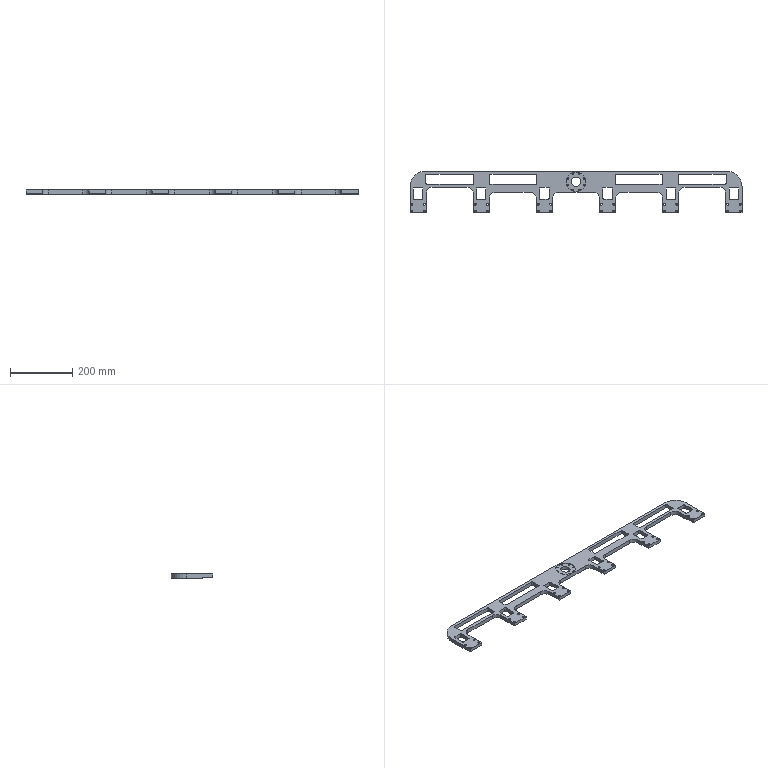NC program | NX | posted with a generic post | part box 1068 x 134 x 13 mm
Lines 126 to 1132 of 9724:
(ZLEVEL_PROFILE_COPY_3 , TOOL : D10)
N232 T10 M6
N234 G54
N236 G17 G0 G90 X130.001 Y-75.258 S9500 M3
N238 G43 Z30. H10
N240 Z4.046
N242 G94 G1 Z-0.954 F1000.
N244 X128.466 Y-72.6
N246 G3 X127.6 Y-72.1 R1.
N248 G1 X75.6 F3500.
N250 G2 X70.5 Y-67. R5.1
N252 G1 Y-20.95
N254 G3 X55.6 Y-6.05 R14.9
N256 G1 X-55.6
N258 G3 X-70.5 Y-20.95 R14.9
N260 G1 Y-67.
N262 G2 X-75.6 Y-72.1 R5.1
N264 G1 X-127.6
N266 G2 X-132.7 Y-67. R5.1
N268 G1 Y-20.95
N270 G3 X-147.6 Y-6.05 R14.9
N272 G1 X-258.8
N274 G3 X-273.7 Y-20.95 R14.9
N276 G1 Y-67.
N278 G2 X-278.8 Y-72.1 R5.1
N280 G1 X-330.8
N282 G2 X-335.9 Y-67. R5.1
N284 G1 Y-5.
N286 G3 X-350.8 Y9.9 R14.9
N288 G1 X-462.
N290 G3 X-476.9 Y-5. R14.9
N292 G1 Y-67.
N294 G2 X-482. Y-72.1 R5.1
N296 G1 X-534.
N298 G2 X-539.1 Y-67. R5.1
N300 G1 Y17.
N302 G2 X-484. Y72.1 R55.1
N304 G1 X127.6
N306 G3 X128.466 Y72.6 R1.
N308 G1 X130.198 Y75.6
N310 Z4.046
N312 G0 Z30.
N314 Z3.092
N316 G1 Z-1.908 F1000.
N318 X128.466 Y72.6
N320 G2 X127.6 Y72.1 R1.
N322 G1 X-484. F3500.
N324 G3 X-539.1 Y17. R55.1
N326 G1 Y-67.
N328 G3 X-534. Y-72.1 R5.1
N330 G1 X-482.
N332 G3 X-476.9 Y-67. R5.1
N334 G1 Y-5.
N336 G2 X-462. Y9.9 R14.9
N338 G1 X-350.8
N340 G2 X-335.9 Y-5. R14.9
N342 G1 Y-67.
N344 G3 X-330.8 Y-72.1 R5.1
N346 G1 X-278.8
N348 G3 X-273.7 Y-67. R5.1
N350 G1 Y-20.95
N352 G2 X-258.8 Y-6.05 R14.9
N354 G1 X-147.6
N356 G2 X-132.7 Y-20.95 R14.9
N358 G1 Y-67.
N360 G3 X-127.6 Y-72.1 R5.1
N362 G1 X-75.6
N364 G3 X-70.5 Y-67. R5.1
N366 G1 Y-20.95
N368 G2 X-55.6 Y-6.05 R14.9
N370 G1 X55.6
N372 G2 X70.5 Y-20.95 R14.9
N374 G1 Y-67.
N376 G3 X75.6 Y-72.1 R5.1
N378 G1 X127.6
N380 G2 X128.466 Y-72.6 R1.
N382 G1 X130.001 Y-75.258
N384 Z3.092
N386 G0 Z30.
N388 Z2.138
N390 G1 Z-2.862 F1000.
N392 X128.466 Y-72.6
N394 G3 X127.6 Y-72.1 R1.
N396 G1 X75.6 F3500.
N398 G2 X70.5 Y-67. R5.1
N400 G1 Y-20.95
N402 G3 X55.6 Y-6.05 R14.9
N404 G1 X-55.6
N406 G3 X-70.5 Y-20.95 R14.9
N408 G1 Y-67.
N410 G2 X-75.6 Y-72.1 R5.1
N412 G1 X-127.6
N414 G2 X-132.7 Y-67. R5.1
N416 G1 Y-20.95
N418 G3 X-147.6 Y-6.05 R14.9
N420 G1 X-258.8
N422 G3 X-273.7 Y-20.95 R14.9
N424 G1 Y-67.
N426 G2 X-278.8 Y-72.1 R5.1
N428 G1 X-330.8
N430 G2 X-335.9 Y-67. R5.1
N432 G1 Y-5.
N434 G3 X-350.8 Y9.9 R14.9
N436 G1 X-462.
N438 G3 X-476.9 Y-5. R14.9
N440 G1 Y-67.
N442 G2 X-482. Y-72.1 R5.1
N444 G1 X-534.
N446 G2 X-539.1 Y-67. R5.1
N448 G1 Y17.
N450 G2 X-484. Y72.1 R55.1
N452 G1 X127.6
N454 G3 X128.466 Y72.6 R1.
N456 G1 X130.198 Y75.6
N458 Z2.138
N460 G0 Z30.
N462 Z1.185
N464 G1 Z-3.815 F1000.
N466 X128.466 Y72.6
N468 G2 X127.6 Y72.1 R1.
N470 G1 X-484. F3500.
N472 G3 X-539.1 Y17. R55.1
N474 G1 Y-67.
N476 G3 X-534. Y-72.1 R5.1
N478 G1 X-482.
N480 G3 X-476.9 Y-67. R5.1
N482 G1 Y-5.
N484 G2 X-462. Y9.9 R14.9
N486 G1 X-350.8
N488 G2 X-335.9 Y-5. R14.9
N490 G1 Y-67.
N492 G3 X-330.8 Y-72.1 R5.1
N494 G1 X-278.8
N496 G3 X-273.7 Y-67. R5.1
N498 G1 Y-20.95
N500 G2 X-258.8 Y-6.05 R14.9
N502 G1 X-147.6
N504 G2 X-132.7 Y-20.95 R14.9
N506 G1 Y-67.
N508 G3 X-127.6 Y-72.1 R5.1
N510 G1 X-75.6
N512 G3 X-70.5 Y-67. R5.1
N514 G1 Y-20.95
N516 G2 X-55.6 Y-6.05 R14.9
N518 G1 X55.6
N520 G2 X70.5 Y-20.95 R14.9
N522 G1 Y-67.
N524 G3 X75.6 Y-72.1 R5.1
N526 G1 X127.6
N528 G2 X128.466 Y-72.6 R1.
N530 G1 X130.001 Y-75.258
N532 Z1.185
N534 G0 Z30.
N536 Z0.231
N538 G1 Z-4.769 F1000.
N540 X128.466 Y-72.6
N542 G3 X127.6 Y-72.1 R1.
N544 G1 X75.6 F3500.
N546 G2 X70.5 Y-67. R5.1
N548 G1 Y-20.95
N550 G3 X55.6 Y-6.05 R14.9
N552 G1 X-55.6
N554 G3 X-70.5 Y-20.95 R14.9
N556 G1 Y-67.
N558 G2 X-75.6 Y-72.1 R5.1
N560 G1 X-127.6
N562 G2 X-132.7 Y-67. R5.1
N564 G1 Y-20.95
N566 G3 X-147.6 Y-6.05 R14.9
N568 G1 X-258.8
N570 G3 X-273.7 Y-20.95 R14.9
N572 G1 Y-67.
N574 G2 X-278.8 Y-72.1 R5.1
N576 G1 X-330.8
N578 G2 X-335.9 Y-67. R5.1
N580 G1 Y-5.
N582 G3 X-350.8 Y9.9 R14.9
N584 G1 X-462.
N586 G3 X-476.9 Y-5. R14.9
N588 G1 Y-67.
N590 G2 X-482. Y-72.1 R5.1
N592 G1 X-534.
N594 G2 X-539.1 Y-67. R5.1
N596 G1 Y17.
N598 G2 X-484. Y72.1 R55.1
N600 G1 X127.6
N602 G3 X128.466 Y72.6 R1.
N604 G1 X130.198 Y75.6
N606 Z0.231
N608 G0 Z30.
N610 Z-0.723
N612 G1 Z-5.723 F1000.
N614 X128.466 Y72.6
N616 G2 X127.6 Y72.1 R1.
N618 G1 X-484. F3500.
N620 G3 X-539.1 Y17. R55.1
N622 G1 Y-67.
N624 G3 X-534. Y-72.1 R5.1
N626 G1 X-482.
N628 G3 X-476.9 Y-67. R5.1
N630 G1 Y-5.
N632 G2 X-462. Y9.9 R14.9
N634 G1 X-350.8
N636 G2 X-335.9 Y-5. R14.9
N638 G1 Y-67.
N640 G3 X-330.8 Y-72.1 R5.1
N642 G1 X-278.8
N644 G3 X-273.7 Y-67. R5.1
N646 G1 Y-20.95
N648 G2 X-258.8 Y-6.05 R14.9
N650 G1 X-147.6
N652 G2 X-132.7 Y-20.95 R14.9
N654 G1 Y-67.
N656 G3 X-127.6 Y-72.1 R5.1
N658 G1 X-75.6
N660 G3 X-70.5 Y-67. R5.1
N662 G1 Y-20.95
N664 G2 X-55.6 Y-6.05 R14.9
N666 G1 X55.6
N668 G2 X70.5 Y-20.95 R14.9
N670 G1 Y-67.
N672 G3 X75.6 Y-72.1 R5.1
N674 G1 X127.6
N676 G2 X128.466 Y-72.6 R1.
N678 G1 X130.001 Y-75.258
N680 Z-0.723
N682 G0 Z30.
N684 Z-1.677
N686 G1 Z-6.677 F1000.
N688 X128.466 Y-72.6
N690 G3 X127.6 Y-72.1 R1.
N692 G1 X75.6 F3500.
N694 G2 X70.5 Y-67. R5.1
N696 G1 Y-20.95
N698 G3 X55.6 Y-6.05 R14.9
N700 G1 X-55.6
N702 G3 X-70.5 Y-20.95 R14.9
N704 G1 Y-67.
N706 G2 X-75.6 Y-72.1 R5.1
N708 G1 X-127.6
N710 G2 X-132.7 Y-67. R5.1
N712 G1 Y-20.95
N714 G3 X-147.6 Y-6.05 R14.9
N716 G1 X-258.8
N718 G3 X-273.7 Y-20.95 R14.9
N720 G1 Y-67.
N722 G2 X-278.8 Y-72.1 R5.1
N724 G1 X-330.8
N726 G2 X-335.9 Y-67. R5.1
N728 G1 Y-5.
N730 G3 X-350.8 Y9.9 R14.9
N732 G1 X-462.
N734 G3 X-476.9 Y-5. R14.9
N736 G1 Y-67.
N738 G2 X-482. Y-72.1 R5.1
N740 G1 X-534.
N742 G2 X-539.1 Y-67. R5.1
N744 G1 Y17.
N746 G2 X-484. Y72.1 R55.1
N748 G1 X127.6
N750 G3 X128.466 Y72.6 R1.
N752 G1 X130.198 Y75.6
N754 Z-1.677
N756 G0 Z30.
N758 Z-2.631
N760 G1 Z-7.631 F1000.
N762 X128.466 Y72.6
N764 G2 X127.6 Y72.1 R1.
N766 G1 X-484. F3500.
N768 G3 X-539.1 Y17. R55.1
N770 G1 Y-67.
N772 G3 X-534. Y-72.1 R5.1
N774 G1 X-482.
N776 G3 X-476.9 Y-67. R5.1
N778 G1 Y-5.
N780 G2 X-462. Y9.9 R14.9
N782 G1 X-350.8
N784 G2 X-335.9 Y-5. R14.9
N786 G1 Y-67.
N788 G3 X-330.8 Y-72.1 R5.1
N790 G1 X-278.8
N792 G3 X-273.7 Y-67. R5.1
N794 G1 Y-20.95
N796 G2 X-258.8 Y-6.05 R14.9
N798 G1 X-147.6
N800 G2 X-132.7 Y-20.95 R14.9
N802 G1 Y-67.
N804 G3 X-127.6 Y-72.1 R5.1
N806 G1 X-75.6
N808 G3 X-70.5 Y-67. R5.1
N810 G1 Y-20.95
N812 G2 X-55.6 Y-6.05 R14.9
N814 G1 X55.6
N816 G2 X70.5 Y-20.95 R14.9
N818 G1 Y-67.
N820 G3 X75.6 Y-72.1 R5.1
N822 G1 X127.6
N824 G2 X128.466 Y-72.6 R1.
N826 G1 X130.001 Y-75.258
N828 Z-2.631
N830 G0 Z30.
N832 Z-3.585
N834 G1 Z-8.585 F1000.
N836 X128.466 Y-72.6
N838 G3 X127.6 Y-72.1 R1.
N840 G1 X75.6 F3500.
N842 G2 X70.5 Y-67. R5.1
N844 G1 Y-20.95
N846 G3 X55.6 Y-6.05 R14.9
N848 G1 X-55.6
N850 G3 X-70.5 Y-20.95 R14.9
N852 G1 Y-67.
N854 G2 X-75.6 Y-72.1 R5.1
N856 G1 X-127.6
N858 G2 X-132.7 Y-67. R5.1
N860 G1 Y-20.95
N862 G3 X-147.6 Y-6.05 R14.9
N864 G1 X-258.8
N866 G3 X-273.7 Y-20.95 R14.9
N868 G1 Y-67.
N870 G2 X-278.8 Y-72.1 R5.1
N872 G1 X-330.8
N874 G2 X-335.9 Y-67. R5.1
N876 G1 Y-5.
N878 G3 X-350.8 Y9.9 R14.9
N880 G1 X-462.
N882 G3 X-476.9 Y-5. R14.9
N884 G1 Y-67.
N886 G2 X-482. Y-72.1 R5.1
N888 G1 X-534.
N890 G2 X-539.1 Y-67. R5.1
N892 G1 Y17.
N894 G2 X-484. Y72.1 R55.1
N896 G1 X127.6
N898 G3 X128.466 Y72.6 R1.
N900 G1 X130.198 Y75.6
N902 Z-3.585
N904 G0 Z30.
N906 Z-4.538
N908 G1 Z-9.538 F1000.
N910 X128.466 Y72.6
N912 G2 X127.6 Y72.1 R1.
N914 G1 X-484. F3500.
N916 G3 X-539.1 Y17. R55.1
N918 G1 Y-67.
N920 G3 X-534. Y-72.1 R5.1
N922 G1 X-482.
N924 G3 X-476.9 Y-67. R5.1
N926 G1 Y-5.
N928 G2 X-462. Y9.9 R14.9
N930 G1 X-350.8
N932 G2 X-335.9 Y-5. R14.9
N934 G1 Y-67.
N936 G3 X-330.8 Y-72.1 R5.1
N938 G1 X-278.8
N940 G3 X-273.7 Y-67. R5.1
N942 G1 Y-20.95
N944 G2 X-258.8 Y-6.05 R14.9
N946 G1 X-147.6
N948 G2 X-132.7 Y-20.95 R14.9
N950 G1 Y-67.
N952 G3 X-127.6 Y-72.1 R5.1
N954 G1 X-75.6
N956 G3 X-70.5 Y-67. R5.1
N958 G1 Y-20.95
N960 G2 X-55.6 Y-6.05 R14.9
N962 G1 X55.6
N964 G2 X70.5 Y-20.95 R14.9
N966 G1 Y-67.
N968 G3 X75.6 Y-72.1 R5.1
N970 G1 X127.6
N972 G2 X128.466 Y-72.6 R1.
N974 G1 X130.001 Y-75.258
N976 Z-4.538
N978 G0 Z30.
N980 Z-5.492
N982 G1 Z-10.492 F1000.
N984 X128.466 Y-72.6
N986 G3 X127.6 Y-72.1 R1.
N988 G1 X75.6 F3500.
N990 G2 X70.5 Y-67. R5.1
N992 G1 Y-20.95
N994 G3 X55.6 Y-6.05 R14.9
N996 G1 X-55.6
N998 G3 X-70.5 Y-20.95 R14.9
N1000 G1 Y-67.
N1002 G2 X-75.6 Y-72.1 R5.1
N1004 G1 X-127.6
N1006 G2 X-132.7 Y-67. R5.1
N1008 G1 Y-20.95
N1010 G3 X-147.6 Y-6.05 R14.9
N1012 G1 X-258.8
N1014 G3 X-273.7 Y-20.95 R14.9
N1016 G1 Y-67.
N1018 G2 X-278.8 Y-72.1 R5.1
N1020 G1 X-330.8
N1022 G2 X-335.9 Y-67. R5.1
N1024 G1 Y-5.
N1026 G3 X-350.8 Y9.9 R14.9
N1028 G1 X-462.
N1030 G3 X-476.9 Y-5. R14.9
N1032 G1 Y-67.
N1034 G2 X-482. Y-72.1 R5.1
N1036 G1 X-534.
N1038 G2 X-539.1 Y-67. R5.1
N1040 G1 Y17.
N1042 G2 X-484. Y72.1 R55.1
N1044 G1 X127.6
N1046 G3 X128.466 Y72.6 R1.
N1048 G1 X130.198 Y75.6
N1050 Z-5.492
N1052 G0 Z30.
N1054 Z-6.446
N1056 G1 Z-11.446 F1000.
N1058 X128.466 Y72.6
N1060 G2 X127.6 Y72.1 R1.
N1062 G1 X-484. F3500.
N1064 G3 X-539.1 Y17. R55.1
N1066 G1 Y-67.
N1068 G3 X-534. Y-72.1 R5.1
N1070 G1 X-482.
N1072 G3 X-476.9 Y-67. R5.1
N1074 G1 Y-5.
N1076 G2 X-462. Y9.9 R14.9
N1078 G1 X-350.8
N1080 G2 X-335.9 Y-5. R14.9
N1082 G1 Y-67.
N1084 G3 X-330.8 Y-72.1 R5.1
N1086 G1 X-278.8
N1088 G3 X-273.7 Y-67. R5.1
N1090 G1 Y-20.95
N1092 G2 X-258.8 Y-6.05 R14.9
N1094 G1 X-147.6
N1096 G2 X-132.7 Y-20.95 R14.9
N1098 G1 Y-67.
N1100 G3 X-127.6 Y-72.1 R5.1
N1102 G1 X-75.6
N1104 G3 X-70.5 Y-67. R5.1
N1106 G1 Y-20.95
N1108 G2 X-55.6 Y-6.05 R14.9
N1110 G1 X55.6
N1112 G2 X70.5 Y-20.95 R14.9
N1114 G1 Y-67.
N1116 G3 X75.6 Y-72.1 R5.1
N1118 G1 X127.6
N1120 G2 X128.466 Y-72.6 R1.
N1122 G1 X130.001 Y-75.258
N1124 Z-6.446
N1126 G0 Z30.
N1128 Z-7.4
N1130 G1 Z-12.4 F1000.
N1132 X128.466 Y-72.6
N1134 G3 X127.6 Y-72.1 R1.
N1136 G1 X75.6 F3500.
N1138 G2 X70.5 Y-67. R5.1
N1140 G1 Y-20.95
N1142 G3 X55.6 Y-6.05 R14.9
N1144 G1 X-55.6
N1146 G3 X-70.5 Y-20.95 R14.9
N1148 G1 Y-67.
N1150 G2 X-75.6 Y-72.1 R5.1
N1152 G1 X-127.6
N1154 G2 X-132.7 Y-67. R5.1
N1156 G1 Y-20.95
N1158 G3 X-147.6 Y-6.05 R14.9
N1160 G1 X-258.8
N1162 G3 X-273.7 Y-20.95 R14.9
N1164 G1 Y-67.
N1166 G2 X-278.8 Y-72.1 R5.1
N1168 G1 X-330.8
N1170 G2 X-335.9 Y-67. R5.1
N1172 G1 Y-5.
N1174 G3 X-350.8 Y9.9 R14.9
N1176 G1 X-462.
N1178 G3 X-476.9 Y-5. R14.9
N1180 G1 Y-67.
N1182 G2 X-482. Y-72.1 R5.1
N1184 G1 X-534.
N1186 G2 X-539.1 Y-67. R5.1
N1188 G1 Y17.
N1190 G2 X-484. Y72.1 R55.1
N1192 G1 X127.6
N1194 G3 X128.466 Y72.6 R1.
N1196 G1 X130.198 Y75.6
N1198 Z-7.4
N1200 G0 Z30.
(ZLEVEL_PROFILE_COPY_2_COPY , TOOL : D10)
N1202 X111.5 Y-1.952
N1204 Z1.5
N1206 G1 Y10.902 Z0.826 F1000.
N1208 X111.453 Y10.9 Z0.824
N1210 X91.747 Z-0.209
N1212 X91.7 Y10.902 Z-0.211
N1214 Y-3.999 Z-0.992
N1216 Y-18.9 F3500.
N1218 X111.5
N1220 Y10.902
N1222 X111.453 Y10.9
N1224 X91.747
N1226 X91.7 Y10.902
N1228 Y-3.999
N1230 Y-18.9 Z-1.252
N1232 X111.5 Z-1.598
N1234 Y3.248 Z-1.985
N1236 Y10.902
N1238 X111.453 Y10.9
N1240 X91.747
N1242 X91.7 Y10.902
N1244 Y-3.999
N1246 Y-18.9 Z-2.245
N1248 X111.5 Z-2.59
N1250 Y3.248 Z-2.977
N1252 Y10.902
N1254 X111.453 Y10.9
N1256 X91.747
N1258 X91.7 Y10.902
N1260 Y-3.999
N1262 Y-18.9 Z-3.237
N1264 X111.5 Z-3.583
N1266 Y3.248 Z-3.969
N1268 Y10.902
N1270 X111.453 Y10.9
N1272 X91.747
N1274 X91.7 Y10.902
N1276 Y-3.999
N1278 Y-18.9 Z-4.229
N1280 X111.5 Z-4.575
N1282 Y3.248 Z-4.962
N1284 Y10.902
N1286 X111.453 Y10.9
N1288 X91.747
N1290 X91.7 Y10.902
N1292 Y-3.999
N1294 Y-18.9 Z-5.222
N1296 X111.5 Z-5.567
N1298 Y3.248 Z-5.954
N1300 Y10.902
N1302 X111.453 Y10.9
N1304 X91.747
N1306 X91.7 Y10.902
N1308 Y-3.999
N1310 Y-18.9 Z-6.214
N1312 X111.5 Z-6.56
N1314 Y3.248 Z-6.946
N1316 Y10.902
N1318 X111.453 Y10.9
N1320 X91.747
N1322 X91.7 Y10.902
N1324 Y-3.999
N1326 Y-18.9 Z-7.206
N1328 X111.5 Z-7.552
N1330 Y3.248 Z-7.938
N1332 Y10.902
N1334 X111.453 Y10.9
N1336 X91.747
N1338 X91.7 Y10.902
N1340 Y-3.999
N1342 Y-18.9 Z-8.199
N1344 X111.5 Z-8.544
N1346 Y3.248 Z-8.931
N1348 Y10.902
N1350 X111.453 Y10.9
N1352 X91.747
N1354 X91.7 Y10.902
N1356 Y-3.999
N1358 Y-18.9 Z-9.191
N1360 X111.5 Z-9.536
N1362 Y3.248 Z-9.923
N1364 Y10.902
N1366 X111.453 Y10.9
N1368 X91.747
N1370 X91.7 Y10.902
N1372 Y-3.999
N1374 Y-18.9 Z-10.183
N1376 X111.5 Z-10.529
N1378 Y3.248 Z-10.915
N1380 Y10.902
N1382 X111.453 Y10.9
N1384 X91.747
N1386 X91.7 Y10.902
N1388 Y-3.999
N1390 Y-18.9 Z-11.175
N1392 X111.5 Z-11.521
N1394 Y3.248 Z-11.908
N1396 Y10.902
N1398 X111.453 Y10.9
N1400 X91.747
N1402 X91.7 Y10.902
N1404 Y-3.999
N1406 Y-18.9 Z-12.168
N1408 X111.5 Z-12.513
N1410 Y3.248 Z-12.9
N1412 Y10.902
N1414 X111.453 Y10.9
N1416 X91.747
N1418 X91.7 Y10.902
N1420 Y-18.9
N1422 X111.5
N1424 Y3.248
N1426 Z-11.4
N1428 G0 Z30.
N1430 X-7.579 Y26.646
N1432 Z1.5
N1434 G1 X-7.38 Y26.401 Z1.483 F1000.
N1436 X-7.166 Y26.161 Z1.467
N1438 X-6.932 Y25.932 Z1.449
N1440 X-6.719 Y25.723 Z1.434
N1442 X-6.484 Y25.519 Z1.418
N1444 X-6.148 Y25.228 Z1.394
N1446 X-5.808 Y24.97 Z1.372
N1448 X-5.433 Y24.724 Z1.348
N1450 X-5.067 Y24.484 Z1.325
N1452 X-4.675 Y24.273 Z1.302
N1454 X-4.283 Y24.063 Z1.279
N1456 X-4.155 Y24.003 Z1.271
N1458 X-3.734 Y23.831 Z1.248
N1460 X-3.322 Y23.663 Z1.224
N1462 X-2.794 Y23.492 Z1.195
N1464 X-2.358 Y23.385 Z1.172
N1466 X-1.926 Y23.279 Z1.148
N1468 X-0.871 Y23.128 Z1.092
N1470 X0.193 Y23.092 Z1.037
N1472 X1.255 Y23.17 Z0.981
N1474 X2.302 Y23.361 Z0.925
N1476 X3.323 Y23.664 Z0.869
N1478 X4.148 Y24. Z0.823
N1480 X5.06 Y24.479 Z0.769
N1482 X5.432 Y24.724 Z0.745
N1484 X6.034 Y25.162 Z0.706
N1486 X6.062 Y25.173 Z0.705
N1488 X6.333 Y25.383 Z0.687
N1490 X6.599 Y25.62 Z0.668
N1492 X6.931 Y25.917 Z0.645
N1494 X7.514 Y26.538 Z0.6
N1496 X8.041 Y27.207 Z0.555
N1498 X8.508 Y27.919 Z0.511
N1500 X8.724 Y28.319 Z0.487
N1502 X8.934 Y28.711 Z0.464
N1504 X9.003 Y28.858 Z0.455
N1506 X9.172 Y29.275 Z0.431
N1508 X9.34 Y29.687 Z0.408
N1510 X9.512 Y30.219 Z0.379
N1512 X9.619 Y30.657 Z0.355
N1514 X9.724 Y31.09 Z0.332
N1516 X9.863 Y32.04 Z0.282
N1518 X9.91 Y33. Z0.231
N1520 X9.863 Y33.96 Z0.181
N1522 X9.724 Y34.91 Z0.13
N1524 X9.617 Y35.348 Z0.107
N1526 X9.512 Y35.781 Z0.084
N1528 X9.34 Y36.313 Z0.054
N1530 X9.168 Y36.737 Z0.03
N1532 X9. Y37.149 Z0.007
N1534 X8.935 Y37.286 Z-0.001
N1536 X8.719 Y37.688 Z-0.025
N1538 X8.509 Y38.08 Z-0.048
N1540 X8.041 Y38.792 Z-0.093
N1542 X7.514 Y39.462 Z-0.138
N1544 X6.931 Y40.083 Z-0.182
N1546 X6.595 Y40.383 Z-0.206
N1548 X6.338 Y40.613 Z-0.224
N1550 X6.057 Y40.831 Z-0.243
N1552 X5.755 Y41.064 Z-0.263
N1554 X5.432 Y41.276 Z-0.283
N1556 X5.06 Y41.521 Z-0.306
N1558 X4.137 Y42.005 Z-0.361
N1560 X3.724 Y42.173 Z-0.384
N1562 X3.311 Y42.34 Z-0.407
N1564 X2.778 Y42.513 Z-0.437
N1566 X2.34 Y42.62 Z-0.46
N1568 X1.907 Y42.725 Z-0.484
N1570 X0.954 Y42.864 Z-0.534
N1572 X-0.009 Y42.91 Z-0.585
N1574 X-0.972 Y42.862 Z-0.635
N1576 X-1.925 Y42.721 Z-0.686
N1578 X-2.361 Y42.614 Z-0.709
N1580 X-2.794 Y42.508 Z-0.733
N1582 X-3.32 Y42.337 Z-0.762
N1584 X-3.742 Y42.165 Z-0.786
N1586 X-4.154 Y41.997 Z-0.809
N1588 X-4.282 Y41.937 Z-0.816
N1590 X-4.681 Y41.723 Z-0.84
N1592 X-5.067 Y41.516 Z-0.863
N1594 X-5.435 Y41.274 Z-0.886
N1596 X-5.807 Y41.03 Z-0.909
N1598 X-6.614 Y40.379 Z-0.964
N1600 X-6.937 Y40.064 Z-0.987
N1602 X-6.97 Y40.031 Z-0.99
N1604 X-7.003 Y39.997 Z-0.992
N1606 G3 X-7.38 Y39.599 R9.9 F3500.
N1608 G1 X-7.822 Y39.057
N1610 X-7.846 Y39.037
N1612 G3 X-9.17 Y36.732 R9.9
N1614 X-9.166 Y29.259 R9.9
N1616 X-8.726 Y28.324 R9.9
N1618 X-8.277 Y27.568 R9.9
N1620 X-7.848 Y26.966 R9.9
N1622 G1 X-7.847 Y26.971
N1624 X-7.841
N1626 X-7.839 Y26.966
N1628 X-7.38 Y26.401
N1630 G3 X-2.358 Y23.385 R9.9
N1632 X5.432 Y24.724 R9.9
N1634 G1 X6.034 Y25.162
N1636 X6.062 Y25.173
N1638 G3 X8.724 Y28.319 R9.9
N1640 X9.168 Y36.737 R9.9
N1642 X6.057 Y40.831 R9.9
N1644 X5.432 Y41.276 R9.9
N1646 X-4.681 Y41.723 R9.9
N1648 X-7.003 Y39.997 R9.9
N1650 G1 X-7.156 Y39.836 Z-0.997
N1652 X-7.305 Y39.671 Z-1.002
N1654 X-7.452 Y39.505 Z-1.006
N1656 X-7.599 Y39.338 Z-1.011
N1658 X-7.737 Y39.165 Z-1.016
N1660 X-7.872 Y38.989 Z-1.021
N1662 X-8.007 Y38.812 Z-1.025
N1664 X-8.136 Y38.632 Z-1.03
N1666 X-8.257 Y38.446 Z-1.035
N1668 X-8.379 Y38.26 Z-1.04
N1670 X-8.498 Y38.073 Z-1.044
N1672 X-8.605 Y37.878 Z-1.049
N1674 X-8.712 Y37.684 Z-1.054
N1676 X-8.82 Y37.489 Z-1.058
N1678 X-8.914 Y37.288 Z-1.063
N1680 X-9.008 Y37.087 Z-1.068
N1682 X-9.101 Y36.885 Z-1.073
N1684 X-9.184 Y36.679 Z-1.077
N1686 X-9.262 Y36.472 Z-1.082
N1688 X-9.341 Y36.264 Z-1.087
N1690 X-9.411 Y36.053 Z-1.092
N1692 X-9.475 Y35.841 Z-1.096
N1694 X-9.537 Y35.627 Z-1.101
N1696 X-9.596 Y35.413 Z-1.106
N1698 X-9.644 Y35.197 Z-1.11
N1700 X-9.693 Y34.98 Z-1.115
N1702 X-9.739 Y34.763 Z-1.12
N1704 X-9.77 Y34.543 Z-1.125
N1706 X-9.803 Y34.323 Z-1.129
N1708 X-9.835 Y34.104 Z-1.134
N1710 X-9.854 Y33.882 Z-1.139
N1712 X-9.869 Y33.661 Z-1.144
N1714 X-9.886 Y33.439 Z-1.148
N1716 X-9.891 Y33.217 Z-1.153
N1718 Y32.995 Z-1.158
N1720 Y32.773 Z-1.162
N1722 X-9.885 Y32.551 Z-1.167
N1724 X-9.869 Y32.33 Z-1.172
N1726 X-9.853 Y32.108 Z-1.177
N1728 X-9.834 Y31.887 Z-1.181
N1730 X-9.801 Y31.667 Z-1.186
N1732 X-9.769 Y31.448 Z-1.191
N1734 X-9.738 Y31.228 Z-1.195
N1736 X-9.689 Y31.011 Z-1.2
N1738 X-9.642 Y30.794 Z-1.205
N1740 X-9.595 Y30.577 Z-1.21
N1742 X-9.535 Y30.363 Z-1.214
N1744 X-9.472 Y30.15 Z-1.219
N1746 X-9.408 Y29.938 Z-1.224
N1748 X-9.338 Y29.727 Z-1.229
N1750 X-9.259 Y29.52 Z-1.233
N1752 X-9.18 Y29.312 Z-1.238
N1754 X-9.097 Y29.106 Z-1.243
N1756 X-9.004 Y28.905 Z-1.247
N1758 X-8.911 Y28.703 Z-1.252
N1760 X-8.816 Y28.502 Z-1.257
N1762 X-8.708 Y28.308 Z-1.262
N1764 X-8.6 Y28.114 Z-1.266
N1766 X-8.493 Y27.919 Z-1.271
N1768 X-8.374 Y27.732 Z-1.276
N1770 X-8.252 Y27.546 Z-1.281
N1772 X-8.131 Y27.361 Z-1.285
N1774 X-8. Y27.181 Z-1.29
N1776 X-7.867 Y27.004 Z-1.295
N1778 X-7.734 Y26.829 Z-1.299
N1780 X-7.596 Y26.658 Z-1.304
N1782 X-7.449 Y26.492 Z-1.309
N1784 X-7.302 Y26.325 Z-1.314
N1786 X-7.152 Y26.162 Z-1.318
N1788 X-6.994 Y26.006 Z-1.323
N1790 X-6.836 Y25.85 Z-1.328
N1792 X-6.678 Y25.694 Z-1.333
N1794 X-6.508 Y25.55 Z-1.337
N1796 X-6.339 Y25.407 Z-1.342
N1798 X-6.169 Y25.263 Z-1.347
N1800 X-5.993 Y25.129 Z-1.351
N1802 X-5.814 Y24.997 Z-1.356
N1804 X-5.635 Y24.866 Z-1.361
N1806 X-5.45 Y24.742 Z-1.366
N1808 X-5.262 Y24.625 Z-1.37
N1810 X-5.073 Y24.508 Z-1.375
N1812 X-4.883 Y24.394 Z-1.38
N1814 X-4.687 Y24.289 Z-1.385
N1816 X-4.491 Y24.185 Z-1.389
N1818 X-4.294 Y24.083 Z-1.394
N1820 X-4.09 Y23.994 Z-1.399
N1822 X-3.887 Y23.904 Z-1.403
N1824 X-3.684 Y23.815 Z-1.408
N1826 X-3.475 Y23.739 Z-1.413
N1828 X-3.266 Y23.663 Z-1.418
N1830 X-3.057 Y23.589 Z-1.422
N1832 X-2.845 Y23.525 Z-1.427
N1834 X-2.633 Y23.457 Z-1.432
N1836 X-2.418 Y23.4 Z-1.436
N1838 X-2.201 Y23.353 Z-1.441
N1840 X-1.983 Y23.31 Z-1.446
N1842 X-1.766 Y23.266 Z-1.451
N1844 X-1.547 Y23.225 Z-1.455
N1846 X-1.327 Y23.198 Z-1.46
N1848 X-1.107 Y23.171 Z-1.465
N1850 X-0.997 Y23.155 Z-1.467
N1852 X-0.886 Y23.14 Z-1.47
N1854 X-0.775 Y23.137 Z-1.472
N1856 X-0.664 Y23.131 Z-1.474
N1858 X-0.443 Y23.118 Z-1.479
N1860 X-0.221 Y23.106 Z-1.484
N1862 X0.001 Y23.1 Z-1.488
N1864 X0.223 Y23.109 Z-1.493
N1866 X0.445 Y23.115 Z-1.498
N1868 X0.667 Y23.129 Z-1.503
N1870 X0.888 Y23.149 Z-1.507
N1872 X1.109 Y23.169 Z-1.512
N1874 X1.329 Y23.194 Z-1.517
N1876 X1.549 Y23.231 Z-1.522
N1878 X1.768 Y23.266 Z-1.526
N1880 X1.986 Y23.305 Z-1.531
N1882 X2.202 Y23.357 Z-1.536
N1884 X2.418 Y23.409 Z-1.54
N1886 X2.634 Y23.46 Z-1.545
N1888 X2.847 Y23.525 Z-1.55
N1890 X3.058 Y23.593 Z-1.555
N1892 X3.269 Y23.661 Z-1.559
N1894 X3.477 Y23.739 Z-1.564
N1896 X3.684 Y23.82 Z-1.569
N1898 X3.89 Y23.903 Z-1.574
N1900 X4.093 Y23.992 Z-1.578
N1902 X4.293 Y24.089 Z-1.583
N1904 X4.493 Y24.186 Z-1.588
N1906 X4.69 Y24.287 Z-1.592
N1908 X4.883 Y24.398 Z-1.597
N1910 X5.075 Y24.51 Z-1.602
N1912 X5.267 Y24.621 Z-1.607
N1914 X5.45 Y24.746 Z-1.611
N1916 X5.634 Y24.871 Z-1.616
N1918 X5.818 Y24.995 Z-1.621
N1920 X5.994 Y25.131 Z-1.625
N1922 X6.168 Y25.268 Z-1.63
N1924 X6.342 Y25.405 Z-1.635
N1926 X6.511 Y25.55 Z-1.64
N1928 X6.674 Y25.7 Z-1.644
N1930 X6.838 Y25.849 Z-1.649
N1932 X6.997 Y26.004 Z-1.654
N1934 X7.15 Y26.165 Z-1.659
N1936 X7.303 Y26.326 Z-1.663
N1938 X7.453 Y26.49 Z-1.668
N1940 X7.594 Y26.662 Z-1.673
N1942 X7.734 Y26.834 Z-1.677
N1944 X7.875 Y27.006 Z-1.682
N1946 X8.003 Y27.187 Z-1.687
N1948 X8.131 Y27.368 Z-1.692
N1950 X8.259 Y27.55 Z-1.696
N1952 X8.377 Y27.738 Z-1.701
N1954 X8.492 Y27.928 Z-1.706
N1956 X8.607 Y28.118 Z-1.711
N1958 X8.713 Y28.313 Z-1.715
N1960 X8.814 Y28.511 Z-1.72
N1962 X8.913 Y28.709 Z-1.725
N1964 X9.01 Y28.909 Z-1.729
N1966 X9.096 Y29.114 Z-1.734
N1968 X9.182 Y29.318 Z-1.739
N1970 X9.267 Y29.524 Z-1.744
N1972 X9.337 Y29.735 Z-1.748
N1974 X9.408 Y29.945 Z-1.753
N1976 X9.479 Y30.155 Z-1.758
N1978 X9.537 Y30.369 Z-1.763
N1980 X9.592 Y30.585 Z-1.767
N1982 X9.648 Y30.8 Z-1.772
N1984 X9.692 Y31.017 Z-1.777
N1986 X9.732 Y31.236 Z-1.781
N1988 X9.772 Y31.454 Z-1.786
N1990 X9.806 Y31.673 Z-1.791
N1992 X9.829 Y31.894 Z-1.796
N1994 X9.854 Y32.115 Z-1.8
N1996 X9.874 Y32.336 Z-1.805
N1998 X9.882 Y32.558 Z-1.81
N2000 X9.889 Y32.78 Z-1.815
N2002 X9.898 Y33.002 Z-1.819
N2004 X9.889 Y33.224 Z-1.824
N2006 X9.881 Y33.446 Z-1.829
N2008 X9.874 Y33.668 Z-1.833
N2010 X9.853 Y33.889 Z-1.838
N2012 X9.829 Y34.109 Z-1.843
N2014 X9.805 Y34.33 Z-1.848
N2016 X9.771 Y34.55 Z-1.852
N2018 X9.731 Y34.768 Z-1.857
N2020 X9.692 Y34.986 Z-1.862
N2022 X9.647 Y35.204 Z-1.866
N2024 X9.591 Y35.419 Z-1.871
N2026 X9.536 Y35.634 Z-1.876
N2028 X9.478 Y35.848 Z-1.881
N2030 X9.407 Y36.059 Z-1.885
N2032 X9.336 Y36.269 Z-1.89
N2034 X9.265 Y36.48 Z-1.895
N2036 X9.181 Y36.685 Z-1.9
N2038 X9.095 Y36.89 Z-1.904
N2040 X9.008 Y37.094 Z-1.909
N2042 X8.912 Y37.294 Z-1.914
N2044 X8.812 Y37.493 Z-1.918
N2046 X8.712 Y37.691 Z-1.923
N2048 X8.605 Y37.885 Z-1.928
N2050 X8.49 Y38.075 Z-1.933
N2052 X8.375 Y38.266 Z-1.937
N2054 X8.257 Y38.453 Z-1.942
N2056 X8.129 Y38.635 Z-1.947
N2058 X8.001 Y38.816 Z-1.952
N2060 X7.872 Y38.997 Z-1.956
N2062 X7.732 Y39.169 Z-1.961
N2064 X7.591 Y39.341 Z-1.966
N2066 X7.452 Y39.514 Z-1.97
N2068 X7.301 Y39.677 Z-1.975
N2070 X7.147 Y39.837 Z-1.98
N2072 X6.998 Y40.002 Z-1.985
N2074 G3 X6.057 Y40.831 R9.9
N2076 X5.432 Y41.276 R9.9
N2078 X-4.681 Y41.723 R9.9
N2080 X-7.003 Y39.997 R9.9
N2082 G1 X-7.156 Y39.836 Z-1.989
N2084 X-7.305 Y39.671 Z-1.994
N2086 X-7.452 Y39.505 Z-1.999
N2088 X-7.599 Y39.338 Z-2.004
N2090 X-7.737 Y39.165 Z-2.008
N2092 X-7.872 Y38.989 Z-2.013
N2094 X-8.007 Y38.812 Z-2.018
N2096 X-8.136 Y38.632 Z-2.022
N2098 X-8.257 Y38.446 Z-2.027
N2100 X-8.379 Y38.26 Z-2.032
N2102 X-8.498 Y38.073 Z-2.037
N2104 X-8.605 Y37.878 Z-2.041
N2106 X-8.712 Y37.684 Z-2.046
N2108 X-8.82 Y37.489 Z-2.051
N2110 X-8.914 Y37.288 Z-2.055
N2112 X-9.008 Y37.087 Z-2.06
N2114 X-9.101 Y36.885 Z-2.065
N2116 X-9.184 Y36.679 Z-2.07
N2118 X-9.262 Y36.472 Z-2.074
N2120 X-9.341 Y36.264 Z-2.079
N2122 X-9.411 Y36.053 Z-2.084
N2124 X-9.475 Y35.841 Z-2.089
N2126 X-9.537 Y35.627 Z-2.093
N2128 X-9.596 Y35.413 Z-2.098
N2130 X-9.644 Y35.197 Z-2.103
N2132 X-9.693 Y34.98 Z-2.107
N2134 X-9.739 Y34.763 Z-2.112
N2136 X-9.77 Y34.543 Z-2.117
N2138 X-9.803 Y34.323 Z-2.122
N2140 X-9.835 Y34.104 Z-2.126
N2142 X-9.854 Y33.882 Z-2.131
N2144 X-9.869 Y33.661 Z-2.136
N2146 X-9.886 Y33.439 Z-2.141
N2148 X-9.891 Y33.217 Z-2.145
N2150 Y32.995 Z-2.15
N2152 Y32.773 Z-2.155
N2154 X-9.885 Y32.551 Z-2.159
N2156 X-9.869 Y32.33 Z-2.164
N2158 X-9.853 Y32.108 Z-2.169
N2160 X-9.834 Y31.887 Z-2.174
N2162 X-9.801 Y31.668 Z-2.178
N2164 X-9.769 Y31.448 Z-2.183
N2166 X-9.738 Y31.228 Z-2.188
N2168 X-9.689 Y31.011 Z-2.193
N2170 X-9.642 Y30.794 Z-2.197
N2172 X-9.595 Y30.577 Z-2.202
N2174 X-9.535 Y30.363 Z-2.207
N2176 X-9.472 Y30.15 Z-2.211
N2178 X-9.408 Y29.938 Z-2.216
N2180 X-9.338 Y29.727 Z-2.221
N2182 X-9.259 Y29.52 Z-2.226
N2184 X-9.18 Y29.312 Z-2.23
N2186 X-9.097 Y29.106 Z-2.235
N2188 X-9.004 Y28.905 Z-2.24
N2190 X-8.911 Y28.703 Z-2.245
N2192 X-8.816 Y28.502 Z-2.249
N2194 X-8.708 Y28.308 Z-2.254
N2196 X-8.6 Y28.114 Z-2.259
N2198 X-8.493 Y27.919 Z-2.263
N2200 X-8.374 Y27.732 Z-2.268
N2202 X-8.252 Y27.546 Z-2.273
N2204 X-8.131 Y27.361 Z-2.278
N2206 X-8. Y27.181 Z-2.282
N2208 X-7.867 Y27.004 Z-2.287
N2210 X-7.734 Y26.829 Z-2.292
N2212 X-7.596 Y26.658 Z-2.296
N2214 X-7.449 Y26.492 Z-2.301
N2216 X-7.302 Y26.325 Z-2.306
N2218 X-7.152 Y26.162 Z-2.311
N2220 X-6.994 Y26.006 Z-2.315
N2222 X-6.836 Y25.85 Z-2.32
N2224 X-6.678 Y25.694 Z-2.325
N2226 X-6.508 Y25.55 Z-2.33
N2228 X-6.339 Y25.407 Z-2.334
N2230 X-6.169 Y25.263 Z-2.339
N2232 X-5.993 Y25.129 Z-2.344